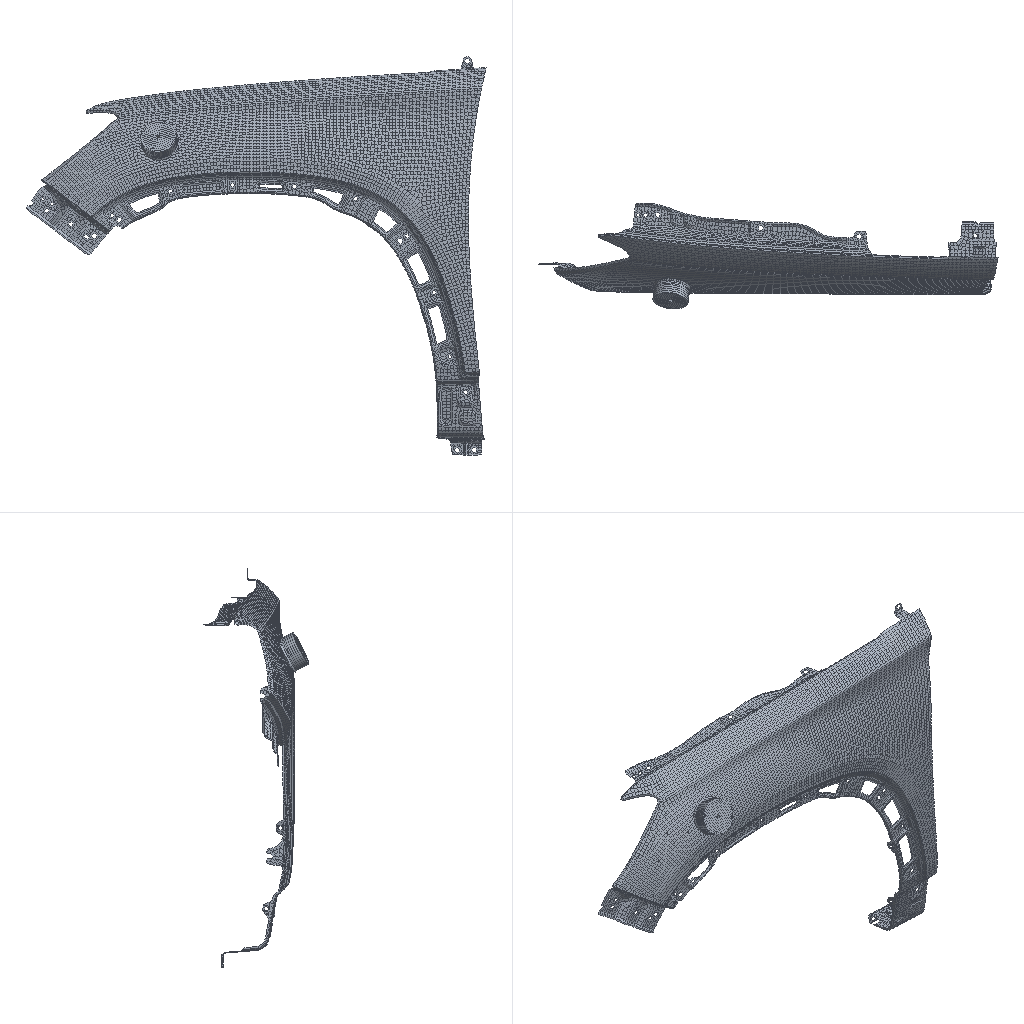Simulation study | abaqus
Set-up summary:
category,name,step,type,value,unit,region
solver,abaqus
solver,version,,,Abaqus/Standard 3DEXPERIENCE R2017x
units,not stated in the deck,,not stated
analysis,deck,,static,static
load_step,load,load,static,nlgeom=True
load_step,unload,unload,static,nlgeom=True
contact,interactions,,,general=0 pairs=1 ties=0
load_step,requested,,,2
mesh,nodes,,,12230
mesh,elements,,,11562
element_type,S3,,shell,568
element_type,S4,,shell,9090
element_type,C3D8,,solid,1664
element_type,C3D8H,,solid,240
load,load commands in deck,,count,3
bc,support commands in deck,,count,14
material,HC180Y,,in results
material,MAT-STEEL,,in results
material,RUBBER,,in results
check,setup vs results,,match,"per instance, exact: element labels, types and connectivity; labels of the nodes the elements use; coordinates not compared"
Abaqus input file, long lists of numbers shortened:
**
** ABAQUS Input Deck Generated by HyperMesh Version  : 14.0.0.88
** Generated using HyperMesh-Abaqus Template Version : 14.0
**
**   Template:  ABAQUS/STANDARD 3D
**
*NODE
         1,  -435.848       ,  -889.15        ,  300.419
         2,  -437.816       ,  -889.15        ,  297.793
** (12228 more lines like these left out)
**HWCOLOR COMP        371    21
*ELEMENT,TYPE=S3,ELSET=KX63_F08-8403101_HC180Y_T070
        13,        27,      3741,      2715
        37,      7291,      7290,       590
** (566 more lines like these left out)
**HWCOLOR COMP        371    21
*ELEMENT,TYPE=S4,ELSET=KX63_F08-8403101_HC180Y_T070
         1,         4,         5,         6,         3
         2,       581,       611,        31,       588
** (9088 more lines like these left out)
**HWCOLOR COMP          1    62
*ELEMENT,TYPE=C3D8,ELSET=impactor
   2127998,    839996,    839958,    840013,    839962,    839818,    839352,    839826,
    839355
** (3326 more lines like these left out)
**HWCOLOR COMP          2    49
*ELEMENT,TYPE=C3D8H,ELSET=rubber
     14376,    838547,    838651,    838694,    838463,    838914,    838951,    839260,
    838890
** (478 more lines like these left out)
**HWNAME COMP    2000070 FRONT_RH_REB2
**HWCOLOR COMP    2000070    58
*KINEMATIC COUPLING,REF NODE=2133045
    838213,1,6
    838215,1,6
    838216,1,6
    838220,1,6
    838224,1,6
    838230,1,6
    838236,1,6
    838237,1,6
    838238,1,6
    838239,1,6
    838242,1,6
    838244,1,6
    838247,1,6
    838248,1,6
    838250,1,6
    838251,1,6
    838252,1,6
    838253,1,6
    838256,1,6
    838257,1,6
    838259,1,6
    838260,1,6
    838272,1,6
    838275,1,6
    838278,1,6
    838282,1,6
    838284,1,6
    838299,1,6
    838301,1,6
    838302,1,6
    838305,1,6
    838307,1,6
    838308,1,6
    838313,1,6
    838315,1,6
    838319,1,6
    838320,1,6
    838321,1,6
    838324,1,6
    838325,1,6
** (224 more lines like these left out)
**HWNAME COMP        370 RB2
**HWCOLOR COMP        370    21
*COUPLING, REF NODE=839102, CONSTRAINT NAME="HM_coupkin_20971", SURFACE="HM_coupkin_surface_20971"
*KINEMATIC
1,6
*SURFACE, NAME ="HM_coupkin_surface_20971", TYPE = NODE
       349, 1
       350, 1
      6702, 1
      6704, 1
      6707, 1
      6709, 1
      6712, 1
      6714, 1
     11735, 1
     11737, 1
     11738, 1
     11741, 1
     11743, 1
     11744, 1
     11754, 1
     11837, 1
     11869, 1
     11870, 1
     11879, 1
     12733, 1
**HWNAME COMP        370 RB2
**HWCOLOR COMP        370    21
*COUPLING, REF NODE=839103, CONSTRAINT NAME="HM_coupkin_20972", SURFACE="HM_coupkin_surface_20972"
*KINEMATIC
1,6
*SURFACE, NAME ="HM_coupkin_surface_20972", TYPE = NODE
       321, 1
       322, 1
      6671, 1
      6678, 1
     12483, 1
     12560, 1
     12561, 1
     12562, 1
     12563, 1
     12568, 1
     12569, 1
     12573, 1
     12574, 1
     12575, 1
     12584, 1
     12585, 1
     12591, 1
     12593, 1
     12600, 1
     12611, 1
**HWNAME COMP        370 RB2
**HWCOLOR COMP        370    21
*COUPLING, REF NODE=839104, CONSTRAINT NAME="HM_coupkin_20973", SURFACE="HM_coupkin_surface_20973"
*KINEMATIC
1,6
*SURFACE, NAME ="HM_coupkin_surface_20973", TYPE = NODE
      7110, 1
      7113, 1
      7118, 1
      7119, 1
      7129, 1
**HWNAME COMP        370 RB2
**HWCOLOR COMP        370    21
*COUPLING, REF NODE=839105, CONSTRAINT NAME="HM_coupkin_20974", SURFACE="HM_coupkin_surface_20974"
*KINEMATIC
1,6
*SURFACE, NAME ="HM_coupkin_surface_20974", TYPE = NODE
     11441, 1
     11445, 1
     11446, 1
     11448, 1
     11451, 1
**HWNAME COMP        370 RB2
**HWCOLOR COMP        370    21
*COUPLING, REF NODE=839106, CONSTRAINT NAME="HM_coupkin_20976", SURFACE="HM_coupkin_surface_20976"
*KINEMATIC
1,6
*SURFACE, NAME ="HM_coupkin_surface_20976", TYPE = NODE
      7300, 1
      7326, 1
      7330, 1
      7331, 1
      7333, 1
      7334, 1
      7335, 1
      7337, 1
     11729, 1
     11749, 1
     11751, 1
     11755, 1
     11756, 1
     11757, 1
     11771, 1
     12043, 1
     12068, 1
     12111, 1
     12116, 1
     12220, 1
**HWNAME COMP        370 RB2
**HWCOLOR COMP        370    21
*COUPLING, REF NODE=839108, CONSTRAINT NAME="HM_coupkin_20983", SURFACE="HM_coupkin_surface_20983"
*KINEMATIC
1,6
*SURFACE, NAME ="HM_coupkin_surface_20983", TYPE = NODE
        36, 1
        49, 1
        78, 1
        80, 1
        81, 1
        82, 1
        85, 1
        91, 1
       105, 1
       107, 1
      7750, 1
      7761, 1
     11457, 1
     11458, 1
     11460, 1
     11461, 1
     11462, 1
     11463, 1
     11464, 1
     11588, 1
    839107, 1
**HWNAME COMP        370 RB2
**HWCOLOR COMP        370    21
*COUPLING, REF NODE=839109, CONSTRAINT NAME="HM_coupkin_20984", SURFACE="HM_coupkin_surface_20984"
*KINEMATIC
1,6
*SURFACE, NAME ="HM_coupkin_surface_20984", TYPE = NODE
      7612, 1
      7613, 1
      7630, 1
     12349, 1
     12580, 1
     12581, 1
     12587, 1
     12588, 1
     12596, 1
     12598, 1
     12601, 1
     12602, 1
     12603, 1
     12604, 1
     12605, 1
     12606, 1
     12607, 1
     12608, 1
     12609, 1
     12610, 1
**HWNAME COMP        370 RB2
**HWCOLOR COMP        370    21
*COUPLING, REF NODE=839110, CONSTRAINT NAME="HM_coupkin_20985", SURFACE="HM_coupkin_surface_20985"
*KINEMATIC
1,6
*SURFACE, NAME ="HM_coupkin_surface_20985", TYPE = NODE
      7451, 1
      7458, 1
     12511, 1
     12514, 1
     12519, 1
     12524, 1
     12525, 1
     12530, 1
     12531, 1
     12536, 1
     12541, 1
     12543, 1
     12546, 1
     12548, 1
     12552, 1
     12553, 1
     12557, 1
     12558, 1
     12576, 1
     12577, 1
**HWNAME COMP        370 RB2
**HWCOLOR COMP        370    21
*COUPLING, REF NODE=839111, CONSTRAINT NAME="HM_coupkin_20986", SURFACE="HM_coupkin_surface_20986"
*KINEMATIC
1,6
*SURFACE, NAME ="HM_coupkin_surface_20986", TYPE = NODE
       675, 1
       677, 1
       678, 1
       682, 1
     12430, 1
     12431, 1
     12435, 1
     12436, 1
     12441, 1
     12442, 1
     12444, 1
     12445, 1
     12446, 1
     12447, 1
     12448, 1
     12449, 1
**HWNAME COMP        370 RB2
**HWCOLOR COMP        370    21
*COUPLING, REF NODE=839144, CONSTRAINT NAME="HM_coupkin_21050", SURFACE="HM_coupkin_surface_21050"
*KINEMATIC
1,6
*SURFACE, NAME ="HM_coupkin_surface_21050", TYPE = NODE
       977, 1
       978, 1
       979, 1
       984, 1
       995, 1
       996, 1
       998, 1
      1018, 1
     12451, 1
     12452, 1
     12453, 1
     12454, 1
     12455, 1
     12456, 1
     12457, 1
     12458, 1
**HWNAME COMP        370 RB2
**HWCOLOR COMP        370    21
*COUPLING, REF NODE=839145, CONSTRAINT NAME="HM_coupkin_21051", SURFACE="HM_coupkin_surface_21051"
*KINEMATIC
1,6
*SURFACE, NAME ="HM_coupkin_surface_21051", TYPE = NODE
       883, 1
       888, 1
       889, 1
       893, 1
       895, 1
       896, 1
       898, 1
       900, 1
       902, 1
       903, 1
       906, 1
       907, 1
       909, 1
       910, 1
       914, 1
     11727, 1
     11775, 1
     11781, 1
     12460, 1
     12463, 1
**HWNAME COMP        370 RB2
**HWCOLOR COMP        370    21
*COUPLING, REF NODE=839146, CONSTRAINT NAME="HM_coupkin_21052", SURFACE="HM_coupkin_surface_21052"
*KINEMATIC
1,6
*SURFACE, NAME ="HM_coupkin_surface_21052", TYPE = NODE
       997, 1
      1008, 1
      1016, 1
      1021, 1
     12078, 1
     12079, 1
     12459, 1
     12461, 1
     12462, 1
     12467, 1
     12468, 1
     12469, 1
**HMNAME SYSTEMCOL auto1,         2,    4
*TRANSFORM, TYPE=R, NSET=HM_auto_transform_208C35
0.994, -0.1045, 0.03226 ,  -0.01827,  -0.4496,  -0.893
**HMORIENT ORIGIN  -205.332,-949.748,512.376
**HM_PROP_ID         38
**HM_comp_by_property "impactor"    56
*SOLID SECTION, ELSET=impactor, MATERIAL=mat-steel
**HM_PROP_ID         39
**HM_comp_by_property "rubber"    56
*SOLID SECTION, ELSET=rubber, MATERIAL=rubber
**HM_PROP_ID         25
**HM_comp_by_property "KX63_F08-8403101_HC180Y_T070"     4
*SHELL SECTION, ELSET=KX63_F08-8403101_HC180Y_T070, MATERIAL=HC180Y
0.7       ,
*ELSET, ELSET=master
      3025,      3029,      3033,      3037,      3041,      3045,      3049,      3053,
      3057,      3061,      3065,      3069,      3073,      3077,      8656,      8668,
** (25 more lines like these left out)
*NSET, NSET=node
   2133045,
*NSET, NSET=HM_auto_transform_208C35
   2133045,
**HMNAME MATS          2 HC180Y     3
*MATERIAL, NAME=HC180Y
*DENSITY
7.8500E-09,0.0
*ELASTIC, TYPE = ISOTROPIC
210000.0  ,0.3       ,0.0
*PLASTIC
239.2     ,0.0       ,0.0
260.6     ,0.0092    ,0.0
281.1     ,0.0149    ,0.0
310.0     ,0.03      ,0.0
329.1     ,0.0431    ,0.0
346.0     ,0.0575    ,0.0
361.8     ,0.074     ,0.0
374.9     ,0.0907    ,0.0
390.9     ,0.115     ,0.0
405.6     ,0.1426    ,0.0
416.3     ,0.1661    ,0.0
423.2     ,0.183     ,0.0
432.6     ,0.2086    ,0.0
439.3     ,0.2298    ,0.0
442.9     ,0.2487    ,0.0
**HMNAME MATS          3 mat-steel     4
*MATERIAL, NAME=mat-steel
*DENSITY
7.8500E-09,0.0
*ELASTIC, TYPE = ISOTROPIC
210000.0  ,0.3       ,0.0
**HMNAME MATS        115 rubber     5
*MATERIAL, NAME=rubber
*DENSITY
1.0000E-09,0.0
*HYPERELASTIC, N = 2,POLYNOMIAL
0.3559   ,-0.2859  ,1.354    ,0.   ,0.   ,0.   ,0.   ,
**HMNAME PROPERTY         40 FRIC
*SURFACE INTERACTION, NAME = FRIC
*FRICTION
0.2       ,0.0       ,0.0       ,0.0
**HMNAME GROUPS         13 cp
*CONTACT PAIR, INTERACTION=FRIC, ADJUST=0.05, TYPE=SURFACE TO SURFACE
slave,master
*SURFACE, NAME = slave, TYPE = ELEMENT
     14376, S2
     14377, S2
    810251, S2
     14378, S2
     14379, S2
     14380, S2
     14385, S2
    810296, S2
     14381, S2
    810252, S2
     14417, S2
     14382, S2
     14387, S2
    810253, S2
     14383, S2
     14384, S2
     14391, S2
     14386, S2
     14388, S2
     14422, S2
     14389, S2
     14390, S2
    810287, S2
     14392, S2
     14496, S2
     14393, S2
     14394, S2
    810267, S2
     14395, S2
     14396, S2
     14397, S2
     14398, S2
     14399, S2
    810254, S2
     14400, S2
     14401, S2
    810255, S2
     14476, S2
     21055, S2
     14402, S2
** (200 more lines like these left out)
*SURFACE, NAME = master, TYPE = ELEMENT
master,SNEG
**HWNAME LOADCOL          1 spc
**HWCOLOR LOADCOL          1    18
*BOUNDARY
    839111,1,6,
    839110,1,6,
    839102,1,6,
    839103,1,6,
    839106,1,6,
    839108,1,6,
    839146,1,6,
    839144,1,6,
    839109,1,6,
    839145,1,6,
    839105,1,6,
    839104,1,6,
   2133045,1,2,
   2133045,4,6,
**HMNAME LOADSTEP          1 load
*STEP, NAME = load, NLGEOM = YES
*STATIC
0.1       ,1.0       ,1.0000E-06,0.2
*MONITOR, DOF =     3, NODE = node
**HWNAME LOADCOL          2 load
**HWCOLOR LOADCOL          2    21
*CLOAD
   2133045,1,2.79
   2133045,2,19.339
   2133045,3,399.522
*OUTPUT, FIELD
*NODE OUTPUT
U,
CF,
*ELEMENT OUTPUT
S,
E,
PEEQ,
*END STEP
**HMNAME LOADSTEP          2 unload
*STEP, NAME = unload, NLGEOM = YES
*STATIC
0.1       ,1.0       ,1.0000E-06,0.2
*MONITOR, DOF =     3, NODE = node
*CLOAD, OP=NEW
*OUTPUT, FIELD
*NODE OUTPUT
U,
CF,
*ELEMENT OUTPUT
S,
E,
PEEQ,
*END STEP
*****
Results summary:
result,step,,completed,increments=15 time=1.0/1.0
result,step,,completed,increments=7 time=1.0/1.0
result,analysis,,,static
result,last_loadstep,,,2
result,analysis steps,,count,2
result,primary field,,,"U, UR"